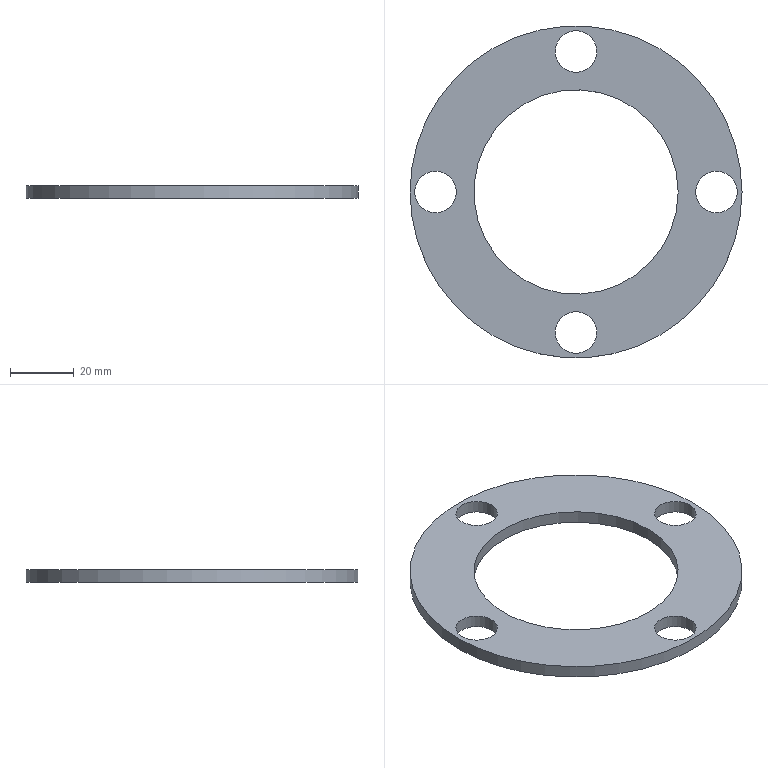Part | NX | features DATUM_CSYS 2, EXTRUDE 1, SKETCH 1 | 1 solid | 8 faces | box 104 x 104 x 4 mm | volume 18988 mm3 | cylinder 6 | plane 2 | commonest cylinder face diameters 13 x4 64 x1 104 x1
STEP:
#1=CARTESIAN_POINT('',(32.,0.,-4.));
#2=VERTEX_POINT('',#1);
#3=CARTESIAN_POINT('',(0.,0.,-4.));
#4=DIRECTION('',(0.,0.,1.));
#5=DIRECTION('',(1.,0.,0.));
#6=AXIS2_PLACEMENT_3D('',#3,#4,#5);
#7=CIRCLE('',#6,32.);
#8=EDGE_CURVE('',#2,#2,#7,.T.);
#9=ORIENTED_EDGE('',*,*,#8,.F.);
#10=EDGE_LOOP('',(#9));
#11=FACE_BOUND('',#10,.T.);
#12=CARTESIAN_POINT('',(32.,0.,0.));
#13=VERTEX_POINT('',#12);
#14=CARTESIAN_POINT('',(0.,0.,0.));
#15=DIRECTION('',(0.,0.,1.));
#16=DIRECTION('',(1.,0.,0.));
#17=AXIS2_PLACEMENT_3D('',#14,#15,#16);
#18=CIRCLE('',#17,32.);
#19=EDGE_CURVE('',#13,#13,#18,.T.);
#20=ORIENTED_EDGE('',*,*,#19,.T.);
#21=EDGE_LOOP('',(#20));
#22=FACE_BOUND('',#21,.T.);
#23=CARTESIAN_POINT('',(0.,0.,-4.));
#24=DIRECTION('',(0.,0.,1.));
#25=DIRECTION('',(1.,0.,0.));
#26=AXIS2_PLACEMENT_3D('',#23,#24,#25);
#27=CYLINDRICAL_SURFACE('',#26,32.);
#28=ADVANCED_FACE('',(#11,#22),#27,.F.);
#29=CARTESIAN_POINT('',(-6.5,-44.,-4.));
#30=VERTEX_POINT('',#29);
#31=CARTESIAN_POINT('',(0.,-44.,-4.));
#32=DIRECTION('',(0.,0.,1.));
#33=DIRECTION('',(-1.,0.,0.));
#34=AXIS2_PLACEMENT_3D('',#31,#32,#33);
#35=CIRCLE('',#34,6.5);
#36=EDGE_CURVE('',#30,#30,#35,.T.);
#37=ORIENTED_EDGE('',*,*,#36,.F.);
#38=EDGE_LOOP('',(#37));
#39=FACE_BOUND('',#38,.T.);
#40=CARTESIAN_POINT('',(-6.5,-44.,0.));
#41=VERTEX_POINT('',#40);
#42=CARTESIAN_POINT('',(0.,-44.,0.));
#43=DIRECTION('',(0.,0.,1.));
#44=DIRECTION('',(-1.,0.,0.));
#45=AXIS2_PLACEMENT_3D('',#42,#43,#44);
#46=CIRCLE('',#45,6.5);
#47=EDGE_CURVE('',#41,#41,#46,.T.);
#48=ORIENTED_EDGE('',*,*,#47,.T.);
#49=EDGE_LOOP('',(#48));
#50=FACE_BOUND('',#49,.T.);
#51=CARTESIAN_POINT('',(0.,-44.,-4.));
#52=DIRECTION('',(0.,0.,1.));
#53=DIRECTION('',(1.,0.,0.));
#54=AXIS2_PLACEMENT_3D('',#51,#52,#53);
#55=CYLINDRICAL_SURFACE('',#54,6.5);
#56=ADVANCED_FACE('',(#39,#50),#55,.F.);
#57=CARTESIAN_POINT('',(6.5,44.,-4.));
#58=VERTEX_POINT('',#57);
#59=CARTESIAN_POINT('',(0.,44.,-4.));
#60=DIRECTION('',(0.,0.,1.));
#61=DIRECTION('',(1.,0.,0.));
#62=AXIS2_PLACEMENT_3D('',#59,#60,#61);
#63=CIRCLE('',#62,6.5);
#64=EDGE_CURVE('',#58,#58,#63,.T.);
#65=ORIENTED_EDGE('',*,*,#64,.F.);
#66=EDGE_LOOP('',(#65));
#67=FACE_BOUND('',#66,.T.);
#68=CARTESIAN_POINT('',(6.5,44.,0.));
#69=VERTEX_POINT('',#68);
#70=CARTESIAN_POINT('',(0.,44.,0.));
#71=DIRECTION('',(0.,0.,1.));
#72=DIRECTION('',(1.,0.,0.));
#73=AXIS2_PLACEMENT_3D('',#70,#71,#72);
#74=CIRCLE('',#73,6.5);
#75=EDGE_CURVE('',#69,#69,#74,.T.);
#76=ORIENTED_EDGE('',*,*,#75,.T.);
#77=EDGE_LOOP('',(#76));
#78=FACE_BOUND('',#77,.T.);
#79=CARTESIAN_POINT('',(0.,44.,-4.));
#80=DIRECTION('',(0.,0.,1.));
#81=DIRECTION('',(1.,0.,0.));
#82=AXIS2_PLACEMENT_3D('',#79,#80,#81);
#83=CYLINDRICAL_SURFACE('',#82,6.5);
#84=ADVANCED_FACE('',(#67,#78),#83,.F.);
#85=CARTESIAN_POINT('',(44.,-6.5,-4.));
#86=VERTEX_POINT('',#85);
#87=CARTESIAN_POINT('',(44.,0.,-4.));
#88=DIRECTION('',(0.,0.,1.));
#89=DIRECTION('',(0.,-1.,0.));
#90=AXIS2_PLACEMENT_3D('',#87,#88,#89);
#91=CIRCLE('',#90,6.5);
#92=EDGE_CURVE('',#86,#86,#91,.T.);
#93=ORIENTED_EDGE('',*,*,#92,.F.);
#94=EDGE_LOOP('',(#93));
#95=FACE_BOUND('',#94,.T.);
#96=CARTESIAN_POINT('',(44.,-6.5,0.));
#97=VERTEX_POINT('',#96);
#98=CARTESIAN_POINT('',(44.,0.,0.));
#99=DIRECTION('',(0.,0.,1.));
#100=DIRECTION('',(0.,-1.,0.));
#101=AXIS2_PLACEMENT_3D('',#98,#99,#100);
#102=CIRCLE('',#101,6.5);
#103=EDGE_CURVE('',#97,#97,#102,.T.);
#104=ORIENTED_EDGE('',*,*,#103,.T.);
#105=EDGE_LOOP('',(#104));
#106=FACE_BOUND('',#105,.T.);
#107=CARTESIAN_POINT('',(44.,0.,-4.));
#108=DIRECTION('',(0.,0.,1.));
#109=DIRECTION('',(1.,0.,0.));
#110=AXIS2_PLACEMENT_3D('',#107,#108,#109);
#111=CYLINDRICAL_SURFACE('',#110,6.5);
#112=ADVANCED_FACE('',(#95,#106),#111,.F.);
#113=CARTESIAN_POINT('',(52.,0.,-4.));
#114=VERTEX_POINT('',#113);
#115=CARTESIAN_POINT('',(0.,0.,-4.));
#116=DIRECTION('',(0.,0.,1.));
#117=DIRECTION('',(1.,0.,0.));
#118=AXIS2_PLACEMENT_3D('',#115,#116,#117);
#119=CIRCLE('',#118,52.);
#120=EDGE_CURVE('',#114,#114,#119,.T.);
#121=ORIENTED_EDGE('',*,*,#120,.T.);
#122=EDGE_LOOP('',(#121));
#123=FACE_BOUND('',#122,.T.);
#124=CARTESIAN_POINT('',(52.,0.,0.));
#125=VERTEX_POINT('',#124);
#126=CARTESIAN_POINT('',(0.,0.,0.));
#127=DIRECTION('',(0.,0.,1.));
#128=DIRECTION('',(1.,0.,0.));
#129=AXIS2_PLACEMENT_3D('',#126,#127,#128);
#130=CIRCLE('',#129,52.);
#131=EDGE_CURVE('',#125,#125,#130,.T.);
#132=ORIENTED_EDGE('',*,*,#131,.F.);
#133=EDGE_LOOP('',(#132));
#134=FACE_BOUND('',#133,.T.);
#135=CARTESIAN_POINT('',(0.,0.,-4.));
#136=DIRECTION('',(0.,0.,1.));
#137=DIRECTION('',(1.,0.,0.));
#138=AXIS2_PLACEMENT_3D('',#135,#136,#137);
#139=CYLINDRICAL_SURFACE('',#138,52.);
#140=ADVANCED_FACE('',(#123,#134),#139,.T.);
#141=CARTESIAN_POINT('',(-44.,6.5,-4.));
#142=VERTEX_POINT('',#141);
#143=CARTESIAN_POINT('',(-44.,0.,-4.));
#144=DIRECTION('',(0.,0.,1.));
#145=DIRECTION('',(0.,1.,0.));
#146=AXIS2_PLACEMENT_3D('',#143,#144,#145);
#147=CIRCLE('',#146,6.5);
#148=EDGE_CURVE('',#142,#142,#147,.T.);
#149=ORIENTED_EDGE('',*,*,#148,.F.);
#150=EDGE_LOOP('',(#149));
#151=FACE_BOUND('',#150,.T.);
#152=CARTESIAN_POINT('',(-44.,6.5,0.));
#153=VERTEX_POINT('',#152);
#154=CARTESIAN_POINT('',(-44.,0.,0.));
#155=DIRECTION('',(0.,0.,1.));
#156=DIRECTION('',(0.,1.,0.));
#157=AXIS2_PLACEMENT_3D('',#154,#155,#156);
#158=CIRCLE('',#157,6.5);
#159=EDGE_CURVE('',#153,#153,#158,.T.);
#160=ORIENTED_EDGE('',*,*,#159,.T.);
#161=EDGE_LOOP('',(#160));
#162=FACE_BOUND('',#161,.T.);
#163=CARTESIAN_POINT('',(-44.,0.,-4.));
#164=DIRECTION('',(0.,0.,1.));
#165=DIRECTION('',(1.,0.,0.));
#166=AXIS2_PLACEMENT_3D('',#163,#164,#165);
#167=CYLINDRICAL_SURFACE('',#166,6.5);
#168=ADVANCED_FACE('',(#151,#162),#167,.F.);
#169=ORIENTED_EDGE('',*,*,#120,.F.);
#170=EDGE_LOOP('',(#169));
#171=FACE_BOUND('',#170,.T.);
#172=ORIENTED_EDGE('',*,*,#92,.T.);
#173=EDGE_LOOP('',(#172));
#174=FACE_BOUND('',#173,.T.);
#175=ORIENTED_EDGE('',*,*,#64,.T.);
#176=EDGE_LOOP('',(#175));
#177=FACE_BOUND('',#176,.T.);
#178=ORIENTED_EDGE('',*,*,#36,.T.);
#179=EDGE_LOOP('',(#178));
#180=FACE_BOUND('',#179,.T.);
#181=ORIENTED_EDGE('',*,*,#8,.T.);
#182=EDGE_LOOP('',(#181));
#183=FACE_BOUND('',#182,.T.);
#184=ORIENTED_EDGE('',*,*,#148,.T.);
#185=EDGE_LOOP('',(#184));
#186=FACE_BOUND('',#185,.T.);
#187=CARTESIAN_POINT('',(22.,0.,-4.));
#188=DIRECTION('',(0.,0.,1.));
#189=DIRECTION('',(1.,0.,0.));
#190=AXIS2_PLACEMENT_3D('',#187,#188,#189);
#191=PLANE('',#190);
#192=ADVANCED_FACE('',(#171,#174,#177,#180,#183,#186),#191,.F.);
#193=ORIENTED_EDGE('',*,*,#131,.T.);
#194=EDGE_LOOP('',(#193));
#195=FACE_BOUND('',#194,.T.);
#196=ORIENTED_EDGE('',*,*,#103,.F.);
#197=EDGE_LOOP('',(#196));
#198=FACE_BOUND('',#197,.T.);
#199=ORIENTED_EDGE('',*,*,#75,.F.);
#200=EDGE_LOOP('',(#199));
#201=FACE_BOUND('',#200,.T.);
#202=ORIENTED_EDGE('',*,*,#47,.F.);
#203=EDGE_LOOP('',(#202));
#204=FACE_BOUND('',#203,.T.);
#205=ORIENTED_EDGE('',*,*,#19,.F.);
#206=EDGE_LOOP('',(#205));
#207=FACE_BOUND('',#206,.T.);
#208=ORIENTED_EDGE('',*,*,#159,.F.);
#209=EDGE_LOOP('',(#208));
#210=FACE_BOUND('',#209,.T.);
#211=CARTESIAN_POINT('',(22.,0.,0.));
#212=DIRECTION('',(0.,0.,1.));
#213=DIRECTION('',(1.,0.,0.));
#214=AXIS2_PLACEMENT_3D('',#211,#212,#213);
#215=PLANE('',#214);
#216=ADVANCED_FACE('',(#195,#198,#201,#204,#207,#210),#215,.T.);
#217=CLOSED_SHELL('',(#28,#56,#84,#112,#140,#168,#192,#216));
#218=MANIFOLD_SOLID_BREP('',#217);
#219=(LENGTH_UNIT()NAMED_UNIT(*)SI_UNIT(.MILLI.,.METRE.));
#220=UNCERTAINTY_MEASURE_WITH_UNIT(LENGTH_MEASURE(0.00001),#219,'','');
#221=(NAMED_UNIT(*)PLANE_ANGLE_UNIT()SI_UNIT($,.RADIAN.));
#222=(NAMED_UNIT(*)SI_UNIT($,.STERADIAN.)SOLID_ANGLE_UNIT());
#223=(GEOMETRIC_REPRESENTATION_CONTEXT(3)GLOBAL_UNCERTAINTY_ASSIGNED_CONTEXT((#220))GLOBAL_UNIT_ASSIGNED_CONTEXT((#219,#221,#222))REPRESENTATION_CONTEXT('',''));
#224=ADVANCED_BREP_SHAPE_REPRESENTATION('',(#218),#223);